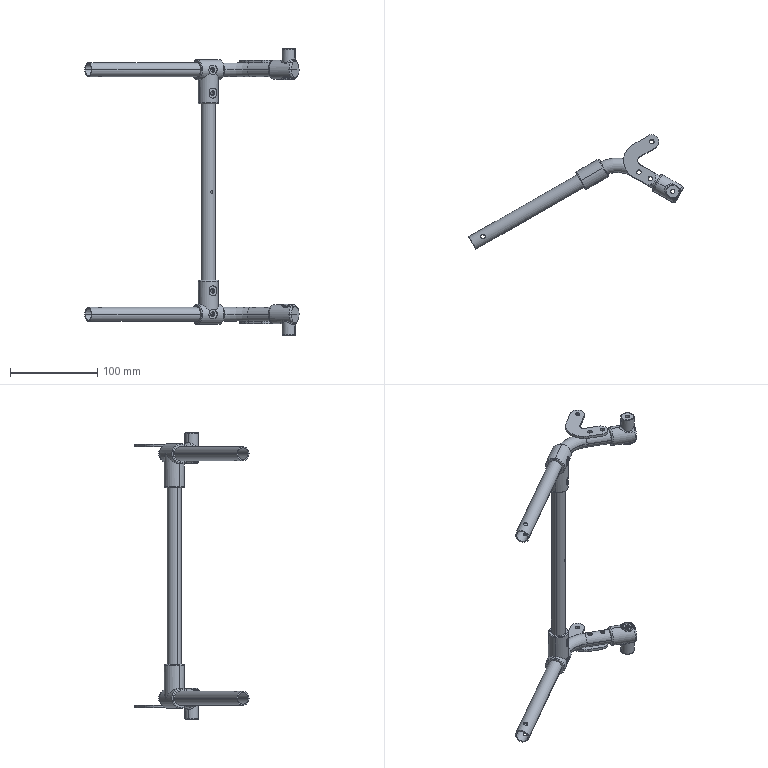Part | SolidWorks | 9 solids | 266 faces | box 245.155 x 130.528 x 328.07 mm | volume 82395 mm3 | cylinder 156 | spline 48 | plane 42 | torus 20 | commonest cylinder face diameters 5.2 x60 16 x14 23 x12 11.2 x10 5.5 x8 13.6 x8